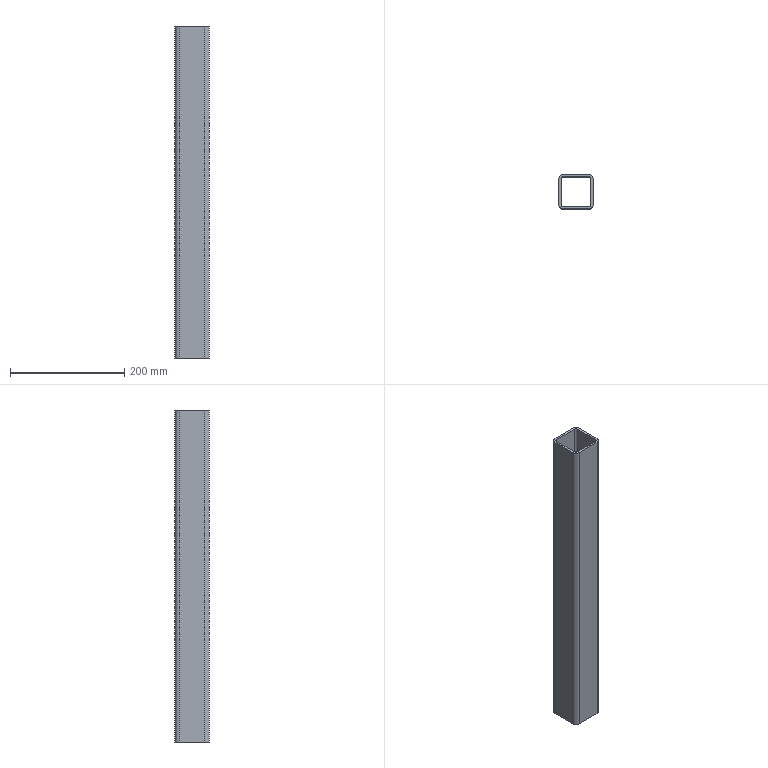Part | SolidWorks | features BaseBody 1 | 1 solid | 18 faces | box 60 x 60 x 580 mm | volume 495782 mm3 | plane 10 | cylinder 8 | commonest cylinder face diameters 8 x4 16 x4
STEP:
#1=CARTESIAN_POINT('',(-692.,1216.,-1300.));
#2=VERTEX_POINT('',#1);
#3=CARTESIAN_POINT('',(-692.,1216.,-720.));
#4=VERTEX_POINT('',#3);
#5=CARTESIAN_POINT('',(-692.,1216.,530.));
#6=DIRECTION('',(0.,0.,1.));
#7=VECTOR('',#6,1000.);
#8=LINE('',#5,#7);
#9=EDGE_CURVE('',#2,#4,#8,.T.);
#10=ORIENTED_EDGE('',*,*,#9,.T.);
#11=CARTESIAN_POINT('',(-648.,1216.,-720.));
#12=VERTEX_POINT('',#11);
#13=CARTESIAN_POINT('',(-692.,1216.,-720.));
#14=DIRECTION('',(1.,0.,0.));
#15=VECTOR('',#14,1000.);
#16=LINE('',#13,#15);
#17=EDGE_CURVE('',#4,#12,#16,.T.);
#18=ORIENTED_EDGE('',*,*,#17,.T.);
#19=CARTESIAN_POINT('',(-648.,1216.,-1300.));
#20=VERTEX_POINT('',#19);
#21=CARTESIAN_POINT('',(-648.,1216.,530.));
#22=DIRECTION('',(0.,0.,-1.));
#23=VECTOR('',#22,1000.);
#24=LINE('',#21,#23);
#25=EDGE_CURVE('',#12,#20,#24,.T.);
#26=ORIENTED_EDGE('',*,*,#25,.T.);
#27=CARTESIAN_POINT('',(-692.,1216.,-1300.));
#28=DIRECTION('',(-1.,0.,0.));
#29=VECTOR('',#28,1000.);
#30=LINE('',#27,#29);
#31=EDGE_CURVE('',#20,#2,#30,.T.);
#32=ORIENTED_EDGE('',*,*,#31,.T.);
#33=EDGE_LOOP('',(#10,#18,#26,#32));
#34=FACE_OUTER_BOUND('',#33,.T.);
#35=CARTESIAN_POINT('',(-692.,1216.,530.));
#36=DIRECTION('',(0.,1.,0.));
#37=DIRECTION('',(0.,0.,1.));
#38=AXIS2_PLACEMENT_3D('',#35,#36,#37);
#39=PLANE('',#38);
#40=ADVANCED_FACE('',(#34),#39,.T.);
#41=CARTESIAN_POINT('',(-696.,1220.,-720.));
#42=VERTEX_POINT('',#41);
#43=CARTESIAN_POINT('',(-692.,1220.,-720.));
#44=DIRECTION('',(0.,0.,1.));
#45=DIRECTION('',(-1.,0.,0.));
#46=AXIS2_PLACEMENT_3D('',#43,#44,#45);
#47=CIRCLE('',#46,4.);
#48=EDGE_CURVE('',#42,#4,#47,.T.);
#49=ORIENTED_EDGE('',*,*,#48,.F.);
#50=CARTESIAN_POINT('',(-696.,1264.,-720.));
#51=VERTEX_POINT('',#50);
#52=CARTESIAN_POINT('',(-696.,1242.,-720.));
#53=DIRECTION('',(0.,-1.,0.));
#54=VECTOR('',#53,1000.);
#55=LINE('',#52,#54);
#56=EDGE_CURVE('',#51,#42,#55,.T.);
#57=ORIENTED_EDGE('',*,*,#56,.F.);
#58=CARTESIAN_POINT('',(-692.,1268.,-720.));
#59=VERTEX_POINT('',#58);
#60=CARTESIAN_POINT('',(-692.,1264.,-720.));
#61=DIRECTION('',(0.,0.,1.));
#62=DIRECTION('',(-1.,0.,0.));
#63=AXIS2_PLACEMENT_3D('',#60,#61,#62);
#64=CIRCLE('',#63,4.);
#65=EDGE_CURVE('',#59,#51,#64,.T.);
#66=ORIENTED_EDGE('',*,*,#65,.F.);
#67=CARTESIAN_POINT('',(-648.,1268.,-720.));
#68=VERTEX_POINT('',#67);
#69=CARTESIAN_POINT('',(0.,1268.,-720.));
#70=DIRECTION('',(-1.,0.,0.));
#71=VECTOR('',#70,1000.);
#72=LINE('',#69,#71);
#73=EDGE_CURVE('',#68,#59,#72,.T.);
#74=ORIENTED_EDGE('',*,*,#73,.F.);
#75=CARTESIAN_POINT('',(-644.,1264.,-720.));
#76=VERTEX_POINT('',#75);
#77=CARTESIAN_POINT('',(-648.,1264.,-720.));
#78=DIRECTION('',(0.,0.,1.));
#79=DIRECTION('',(-1.,0.,0.));
#80=AXIS2_PLACEMENT_3D('',#77,#78,#79);
#81=CIRCLE('',#80,4.);
#82=EDGE_CURVE('',#76,#68,#81,.T.);
#83=ORIENTED_EDGE('',*,*,#82,.F.);
#84=CARTESIAN_POINT('',(-644.,1220.,-720.));
#85=VERTEX_POINT('',#84);
#86=CARTESIAN_POINT('',(-644.,1242.,-720.));
#87=DIRECTION('',(0.,1.,0.));
#88=VECTOR('',#87,1000.);
#89=LINE('',#86,#88);
#90=EDGE_CURVE('',#85,#76,#89,.T.);
#91=ORIENTED_EDGE('',*,*,#90,.F.);
#92=CARTESIAN_POINT('',(-648.,1220.,-720.));
#93=DIRECTION('',(0.,0.,1.));
#94=DIRECTION('',(-1.,0.,0.));
#95=AXIS2_PLACEMENT_3D('',#92,#93,#94);
#96=CIRCLE('',#95,4.);
#97=EDGE_CURVE('',#12,#85,#96,.T.);
#98=ORIENTED_EDGE('',*,*,#97,.F.);
#99=ORIENTED_EDGE('',*,*,#17,.F.);
#100=EDGE_LOOP('',(#49,#57,#66,#74,#83,#91,#98,#99));
#101=FACE_BOUND('',#100,.T.);
#102=CARTESIAN_POINT('',(-640.,1264.,-720.));
#103=VERTEX_POINT('',#102);
#104=CARTESIAN_POINT('',(-640.,1220.,-720.));
#105=VERTEX_POINT('',#104);
#106=CARTESIAN_POINT('',(-640.,1242.,-720.));
#107=DIRECTION('',(0.,-1.,0.));
#108=VECTOR('',#107,1000.);
#109=LINE('',#106,#108);
#110=EDGE_CURVE('',#103,#105,#109,.T.);
#111=ORIENTED_EDGE('',*,*,#110,.F.);
#112=CARTESIAN_POINT('',(-648.,1272.,-720.));
#113=VERTEX_POINT('',#112);
#114=CARTESIAN_POINT('',(-648.,1264.,-720.));
#115=DIRECTION('',(0.,0.,-1.));
#116=DIRECTION('',(-1.,0.,0.));
#117=AXIS2_PLACEMENT_3D('',#114,#115,#116);
#118=CIRCLE('',#117,8.);
#119=EDGE_CURVE('',#113,#103,#118,.T.);
#120=ORIENTED_EDGE('',*,*,#119,.F.);
#121=CARTESIAN_POINT('',(-692.,1272.,-720.));
#122=VERTEX_POINT('',#121);
#123=CARTESIAN_POINT('',(0.,1272.,-720.));
#124=DIRECTION('',(1.,0.,0.));
#125=VECTOR('',#124,1000.);
#126=LINE('',#123,#125);
#127=EDGE_CURVE('',#122,#113,#126,.T.);
#128=ORIENTED_EDGE('',*,*,#127,.F.);
#129=CARTESIAN_POINT('',(-700.,1264.,-720.));
#130=VERTEX_POINT('',#129);
#131=CARTESIAN_POINT('',(-692.,1264.,-720.));
#132=DIRECTION('',(0.,0.,-1.));
#133=DIRECTION('',(-1.,0.,0.));
#134=AXIS2_PLACEMENT_3D('',#131,#132,#133);
#135=CIRCLE('',#134,8.);
#136=EDGE_CURVE('',#130,#122,#135,.T.);
#137=ORIENTED_EDGE('',*,*,#136,.F.);
#138=CARTESIAN_POINT('',(-700.,1220.,-720.));
#139=VERTEX_POINT('',#138);
#140=CARTESIAN_POINT('',(-700.,1242.,-720.));
#141=DIRECTION('',(0.,1.,0.));
#142=VECTOR('',#141,1000.);
#143=LINE('',#140,#142);
#144=EDGE_CURVE('',#139,#130,#143,.T.);
#145=ORIENTED_EDGE('',*,*,#144,.F.);
#146=CARTESIAN_POINT('',(-692.,1212.,-720.));
#147=VERTEX_POINT('',#146);
#148=CARTESIAN_POINT('',(-692.,1220.,-720.));
#149=DIRECTION('',(0.,0.,-1.));
#150=DIRECTION('',(-1.,0.,0.));
#151=AXIS2_PLACEMENT_3D('',#148,#149,#150);
#152=CIRCLE('',#151,8.);
#153=EDGE_CURVE('',#147,#139,#152,.T.);
#154=ORIENTED_EDGE('',*,*,#153,.F.);
#155=CARTESIAN_POINT('',(-648.,1212.,-720.));
#156=VERTEX_POINT('',#155);
#157=CARTESIAN_POINT('',(0.,1212.,-720.));
#158=DIRECTION('',(-1.,0.,0.));
#159=VECTOR('',#158,1000.);
#160=LINE('',#157,#159);
#161=EDGE_CURVE('',#156,#147,#160,.T.);
#162=ORIENTED_EDGE('',*,*,#161,.F.);
#163=CARTESIAN_POINT('',(-648.,1220.,-720.));
#164=DIRECTION('',(0.,0.,-1.));
#165=DIRECTION('',(-1.,0.,0.));
#166=AXIS2_PLACEMENT_3D('',#163,#164,#165);
#167=CIRCLE('',#166,8.);
#168=EDGE_CURVE('',#105,#156,#167,.T.);
#169=ORIENTED_EDGE('',*,*,#168,.F.);
#170=EDGE_LOOP('',(#111,#120,#128,#137,#145,#154,#162,#169));
#171=FACE_OUTER_BOUND('',#170,.T.);
#172=CARTESIAN_POINT('',(0.,1242.,-720.));
#173=DIRECTION('',(0.,0.,-1.));
#174=DIRECTION('',(-1.,0.,0.));
#175=AXIS2_PLACEMENT_3D('',#172,#173,#174);
#176=PLANE('',#175);
#177=ADVANCED_FACE('',(#101,#171),#176,.F.);
#178=CARTESIAN_POINT('',(-696.,1220.,-1300.));
#179=VERTEX_POINT('',#178);
#180=CARTESIAN_POINT('',(-692.,1220.,-1300.));
#181=DIRECTION('',(0.,0.,1.));
#182=DIRECTION('',(-1.,0.,0.));
#183=AXIS2_PLACEMENT_3D('',#180,#181,#182);
#184=CIRCLE('',#183,4.);
#185=EDGE_CURVE('',#179,#2,#184,.T.);
#186=ORIENTED_EDGE('',*,*,#185,.F.);
#187=CARTESIAN_POINT('',(-696.,1220.,530.));
#188=DIRECTION('',(0.,0.,-1.));
#189=VECTOR('',#188,1000.);
#190=LINE('',#187,#189);
#191=EDGE_CURVE('',#42,#179,#190,.T.);
#192=ORIENTED_EDGE('',*,*,#191,.F.);
#193=ORIENTED_EDGE('',*,*,#48,.T.);
#194=ORIENTED_EDGE('',*,*,#9,.F.);
#195=EDGE_LOOP('',(#186,#192,#193,#194));
#196=FACE_OUTER_BOUND('',#195,.T.);
#197=CARTESIAN_POINT('',(-692.,1220.,530.));
#198=DIRECTION('',(0.,0.,-1.));
#199=DIRECTION('',(-1.,0.,0.));
#200=AXIS2_PLACEMENT_3D('',#197,#198,#199);
#201=CYLINDRICAL_SURFACE('',#200,4.);
#202=ADVANCED_FACE('',(#196),#201,.F.);
#203=ORIENTED_EDGE('',*,*,#31,.F.);
#204=CARTESIAN_POINT('',(-644.,1220.,-1300.));
#205=VERTEX_POINT('',#204);
#206=CARTESIAN_POINT('',(-648.,1220.,-1300.));
#207=DIRECTION('',(0.,0.,1.));
#208=DIRECTION('',(-1.,0.,0.));
#209=AXIS2_PLACEMENT_3D('',#206,#207,#208);
#210=CIRCLE('',#209,4.);
#211=EDGE_CURVE('',#20,#205,#210,.T.);
#212=ORIENTED_EDGE('',*,*,#211,.T.);
#213=CARTESIAN_POINT('',(-644.,1264.,-1300.));
#214=VERTEX_POINT('',#213);
#215=CARTESIAN_POINT('',(-644.,1242.,-1300.));
#216=DIRECTION('',(0.,1.,0.));
#217=VECTOR('',#216,1000.);
#218=LINE('',#215,#217);
#219=EDGE_CURVE('',#205,#214,#218,.T.);
#220=ORIENTED_EDGE('',*,*,#219,.T.);
#221=CARTESIAN_POINT('',(-648.,1268.,-1300.));
#222=VERTEX_POINT('',#221);
#223=CARTESIAN_POINT('',(-648.,1264.,-1300.));
#224=DIRECTION('',(0.,0.,1.));
#225=DIRECTION('',(-1.,0.,0.));
#226=AXIS2_PLACEMENT_3D('',#223,#224,#225);
#227=CIRCLE('',#226,4.);
#228=EDGE_CURVE('',#214,#222,#227,.T.);
#229=ORIENTED_EDGE('',*,*,#228,.T.);
#230=CARTESIAN_POINT('',(-692.,1268.,-1300.));
#231=VERTEX_POINT('',#230);
#232=CARTESIAN_POINT('',(-700.,1268.,-1300.));
#233=DIRECTION('',(-1.,0.,0.));
#234=VECTOR('',#233,1000.);
#235=LINE('',#232,#234);
#236=EDGE_CURVE('',#222,#231,#235,.T.);
#237=ORIENTED_EDGE('',*,*,#236,.T.);
#238=CARTESIAN_POINT('',(-696.,1264.,-1300.));
#239=VERTEX_POINT('',#238);
#240=CARTESIAN_POINT('',(-692.,1264.,-1300.));
#241=DIRECTION('',(0.,0.,1.));
#242=DIRECTION('',(-1.,0.,0.));
#243=AXIS2_PLACEMENT_3D('',#240,#241,#242);
#244=CIRCLE('',#243,4.);
#245=EDGE_CURVE('',#231,#239,#244,.T.);
#246=ORIENTED_EDGE('',*,*,#245,.T.);
#247=CARTESIAN_POINT('',(-696.,1242.,-1300.));
#248=DIRECTION('',(0.,-1.,0.));
#249=VECTOR('',#248,1000.);
#250=LINE('',#247,#249);
#251=EDGE_CURVE('',#239,#179,#250,.T.);
#252=ORIENTED_EDGE('',*,*,#251,.T.);
#253=ORIENTED_EDGE('',*,*,#185,.T.);
#254=EDGE_LOOP('',(#203,#212,#220,#229,#237,#246,#252,#253));
#255=FACE_BOUND('',#254,.T.);
#256=CARTESIAN_POINT('',(-640.,1220.,-1300.));
#257=VERTEX_POINT('',#256);
#258=CARTESIAN_POINT('',(-648.,1212.,-1300.));
#259=VERTEX_POINT('',#258);
#260=CARTESIAN_POINT('',(-648.,1220.,-1300.));
#261=DIRECTION('',(0.,0.,-1.));
#262=DIRECTION('',(-1.,0.,0.));
#263=AXIS2_PLACEMENT_3D('',#260,#261,#262);
#264=CIRCLE('',#263,8.);
#265=EDGE_CURVE('',#257,#259,#264,.T.);
#266=ORIENTED_EDGE('',*,*,#265,.T.);
#267=CARTESIAN_POINT('',(-692.,1212.,-1300.));
#268=VERTEX_POINT('',#267);
#269=CARTESIAN_POINT('',(-700.,1212.,-1300.));
#270=DIRECTION('',(-1.,0.,0.));
#271=VECTOR('',#270,1000.);
#272=LINE('',#269,#271);
#273=EDGE_CURVE('',#259,#268,#272,.T.);
#274=ORIENTED_EDGE('',*,*,#273,.T.);
#275=CARTESIAN_POINT('',(-700.,1220.,-1300.));
#276=VERTEX_POINT('',#275);
#277=CARTESIAN_POINT('',(-692.,1220.,-1300.));
#278=DIRECTION('',(0.,0.,-1.));
#279=DIRECTION('',(-1.,0.,0.));
#280=AXIS2_PLACEMENT_3D('',#277,#278,#279);
#281=CIRCLE('',#280,8.);
#282=EDGE_CURVE('',#268,#276,#281,.T.);
#283=ORIENTED_EDGE('',*,*,#282,.T.);
#284=CARTESIAN_POINT('',(-700.,1264.,-1300.));
#285=VERTEX_POINT('',#284);
#286=CARTESIAN_POINT('',(-700.,1242.,-1300.));
#287=DIRECTION('',(0.,1.,0.));
#288=VECTOR('',#287,1000.);
#289=LINE('',#286,#288);
#290=EDGE_CURVE('',#276,#285,#289,.T.);
#291=ORIENTED_EDGE('',*,*,#290,.T.);
#292=CARTESIAN_POINT('',(-692.,1272.,-1300.));
#293=VERTEX_POINT('',#292);
#294=CARTESIAN_POINT('',(-692.,1264.,-1300.));
#295=DIRECTION('',(0.,0.,-1.));
#296=DIRECTION('',(-1.,0.,0.));
#297=AXIS2_PLACEMENT_3D('',#294,#295,#296);
#298=CIRCLE('',#297,8.);
#299=EDGE_CURVE('',#285,#293,#298,.T.);
#300=ORIENTED_EDGE('',*,*,#299,.T.);
#301=CARTESIAN_POINT('',(-648.,1272.,-1300.));
#302=VERTEX_POINT('',#301);
#303=CARTESIAN_POINT('',(-700.,1272.,-1300.));
#304=DIRECTION('',(1.,0.,0.));
#305=VECTOR('',#304,1000.);
#306=LINE('',#303,#305);
#307=EDGE_CURVE('',#293,#302,#306,.T.);
#308=ORIENTED_EDGE('',*,*,#307,.T.);
#309=CARTESIAN_POINT('',(-640.,1264.,-1300.));
#310=VERTEX_POINT('',#309);
#311=CARTESIAN_POINT('',(-648.,1264.,-1300.));
#312=DIRECTION('',(0.,0.,-1.));
#313=DIRECTION('',(-1.,0.,0.));
#314=AXIS2_PLACEMENT_3D('',#311,#312,#313);
#315=CIRCLE('',#314,8.);
#316=EDGE_CURVE('',#302,#310,#315,.T.);
#317=ORIENTED_EDGE('',*,*,#316,.T.);
#318=CARTESIAN_POINT('',(-640.,1242.,-1300.));
#319=DIRECTION('',(0.,-1.,0.));
#320=VECTOR('',#319,1000.);
#321=LINE('',#318,#320);
#322=EDGE_CURVE('',#310,#257,#321,.T.);
#323=ORIENTED_EDGE('',*,*,#322,.T.);
#324=EDGE_LOOP('',(#266,#274,#283,#291,#300,#308,#317,#323));
#325=FACE_OUTER_BOUND('',#324,.T.);
#326=CARTESIAN_POINT('',(-700.,1242.,-1300.));
#327=DIRECTION('',(0.,0.,-1.));
#328=DIRECTION('',(-1.,0.,0.));
#329=AXIS2_PLACEMENT_3D('',#326,#327,#328);
#330=PLANE('',#329);
#331=ADVANCED_FACE('',(#255,#325),#330,.T.);
#332=ORIENTED_EDGE('',*,*,#211,.F.);
#333=ORIENTED_EDGE('',*,*,#25,.F.);
#334=ORIENTED_EDGE('',*,*,#97,.T.);
#335=CARTESIAN_POINT('',(-644.,1220.,530.));
#336=DIRECTION('',(0.,0.,1.));
#337=VECTOR('',#336,1000.);
#338=LINE('',#335,#337);
#339=EDGE_CURVE('',#205,#85,#338,.T.);
#340=ORIENTED_EDGE('',*,*,#339,.F.);
#341=EDGE_LOOP('',(#332,#333,#334,#340));
#342=FACE_OUTER_BOUND('',#341,.T.);
#343=CARTESIAN_POINT('',(-648.,1220.,530.));
#344=DIRECTION('',(0.,0.,-1.));
#345=DIRECTION('',(-1.,0.,0.));
#346=AXIS2_PLACEMENT_3D('',#343,#344,#345);
#347=CYLINDRICAL_SURFACE('',#346,4.);
#348=ADVANCED_FACE('',(#342),#347,.F.);
#349=CARTESIAN_POINT('',(-696.,1264.,530.));
#350=DIRECTION('',(0.,0.,1.));
#351=VECTOR('',#350,1000.);
#352=LINE('',#349,#351);
#353=EDGE_CURVE('',#239,#51,#352,.T.);
#354=ORIENTED_EDGE('',*,*,#353,.T.);
#355=ORIENTED_EDGE('',*,*,#56,.T.);
#356=ORIENTED_EDGE('',*,*,#191,.T.);
#357=ORIENTED_EDGE('',*,*,#251,.F.);
#358=EDGE_LOOP('',(#354,#355,#356,#357));
#359=FACE_OUTER_BOUND('',#358,.T.);
#360=CARTESIAN_POINT('',(-696.,1220.,530.));
#361=DIRECTION('',(1.,0.,0.));
#362=DIRECTION('',(0.,0.,-1.));
#363=AXIS2_PLACEMENT_3D('',#360,#361,#362);
#364=PLANE('',#363);
#365=ADVANCED_FACE('',(#359),#364,.T.);
#366=ORIENTED_EDGE('',*,*,#245,.F.);
#367=CARTESIAN_POINT('',(-692.,1268.,530.));
#368=DIRECTION('',(0.,0.,-1.));
#369=VECTOR('',#368,1000.);
#370=LINE('',#367,#369);
#371=EDGE_CURVE('',#59,#231,#370,.T.);
#372=ORIENTED_EDGE('',*,*,#371,.F.);
#373=ORIENTED_EDGE('',*,*,#65,.T.);
#374=ORIENTED_EDGE('',*,*,#353,.F.);
#375=EDGE_LOOP('',(#366,#372,#373,#374));
#376=FACE_OUTER_BOUND('',#375,.T.);
#377=CARTESIAN_POINT('',(-692.,1264.,530.));
#378=DIRECTION('',(0.,0.,-1.));
#379=DIRECTION('',(-1.,0.,0.));
#380=AXIS2_PLACEMENT_3D('',#377,#378,#379);
#381=CYLINDRICAL_SURFACE('',#380,4.);
#382=ADVANCED_FACE('',(#376),#381,.F.);
#383=CARTESIAN_POINT('',(-648.,1268.,530.));
#384=DIRECTION('',(0.,0.,1.));
#385=VECTOR('',#384,1000.);
#386=LINE('',#383,#385);
#387=EDGE_CURVE('',#222,#68,#386,.T.);
#388=ORIENTED_EDGE('',*,*,#387,.T.);
#389=ORIENTED_EDGE('',*,*,#73,.T.);
#390=ORIENTED_EDGE('',*,*,#371,.T.);
#391=ORIENTED_EDGE('',*,*,#236,.F.);
#392=EDGE_LOOP('',(#388,#389,#390,#391));
#393=FACE_OUTER_BOUND('',#392,.T.);
#394=CARTESIAN_POINT('',(-648.,1268.,530.));
#395=DIRECTION('',(0.,-1.,0.));
#396=DIRECTION('',(0.,0.,-1.));
#397=AXIS2_PLACEMENT_3D('',#394,#395,#396);
#398=PLANE('',#397);
#399=ADVANCED_FACE('',(#393),#398,.T.);
#400=ORIENTED_EDGE('',*,*,#228,.F.);
#401=CARTESIAN_POINT('',(-644.,1264.,530.));
#402=DIRECTION('',(0.,0.,-1.));
#403=VECTOR('',#402,1000.);
#404=LINE('',#401,#403);
#405=EDGE_CURVE('',#76,#214,#404,.T.);
#406=ORIENTED_EDGE('',*,*,#405,.F.);
#407=ORIENTED_EDGE('',*,*,#82,.T.);
#408=ORIENTED_EDGE('',*,*,#387,.F.);
#409=EDGE_LOOP('',(#400,#406,#407,#408));
#410=FACE_OUTER_BOUND('',#409,.T.);
#411=CARTESIAN_POINT('',(-648.,1264.,530.));
#412=DIRECTION('',(0.,0.,-1.));
#413=DIRECTION('',(-1.,0.,0.));
#414=AXIS2_PLACEMENT_3D('',#411,#412,#413);
#415=CYLINDRICAL_SURFACE('',#414,4.);
#416=ADVANCED_FACE('',(#410),#415,.F.);
#417=ORIENTED_EDGE('',*,*,#339,.T.);
#418=ORIENTED_EDGE('',*,*,#90,.T.);
#419=ORIENTED_EDGE('',*,*,#405,.T.);
#420=ORIENTED_EDGE('',*,*,#219,.F.);
#421=EDGE_LOOP('',(#417,#418,#419,#420));
#422=FACE_OUTER_BOUND('',#421,.T.);
#423=CARTESIAN_POINT('',(-644.,1264.,530.));
#424=DIRECTION('',(-1.,0.,0.));
#425=DIRECTION('',(0.,0.,1.));
#426=AXIS2_PLACEMENT_3D('',#423,#424,#425);
#427=PLANE('',#426);
#428=ADVANCED_FACE('',(#422),#427,.T.);
#429=ORIENTED_EDGE('',*,*,#265,.F.);
#430=CARTESIAN_POINT('',(-640.,1220.,530.));
#431=DIRECTION('',(0.,0.,1.));
#432=VECTOR('',#431,1000.);
#433=LINE('',#430,#432);
#434=EDGE_CURVE('',#257,#105,#433,.T.);
#435=ORIENTED_EDGE('',*,*,#434,.T.);
#436=ORIENTED_EDGE('',*,*,#168,.T.);
#437=CARTESIAN_POINT('',(-648.,1212.,530.));
#438=DIRECTION('',(0.,0.,-1.));
#439=VECTOR('',#438,1000.);
#440=LINE('',#437,#439);
#441=EDGE_CURVE('',#156,#259,#440,.T.);
#442=ORIENTED_EDGE('',*,*,#441,.T.);
#443=EDGE_LOOP('',(#429,#435,#436,#442));
#444=FACE_OUTER_BOUND('',#443,.T.);
#445=CARTESIAN_POINT('',(-648.,1220.,530.));
#446=DIRECTION('',(0.,0.,-1.));
#447=DIRECTION('',(-1.,0.,0.));
#448=AXIS2_PLACEMENT_3D('',#445,#446,#447);
#449=CYLINDRICAL_SURFACE('',#448,8.);
#450=ADVANCED_FACE('',(#444),#449,.T.);
#451=ORIENTED_EDGE('',*,*,#434,.F.);
#452=ORIENTED_EDGE('',*,*,#322,.F.);
#453=CARTESIAN_POINT('',(-640.,1264.,530.));
#454=DIRECTION('',(0.,0.,-1.));
#455=VECTOR('',#454,1000.);
#456=LINE('',#453,#455);
#457=EDGE_CURVE('',#103,#310,#456,.T.);
#458=ORIENTED_EDGE('',*,*,#457,.F.);
#459=ORIENTED_EDGE('',*,*,#110,.T.);
#460=EDGE_LOOP('',(#451,#452,#458,#459));
#461=FACE_OUTER_BOUND('',#460,.T.);
#462=CARTESIAN_POINT('',(-640.,1264.,530.));
#463=DIRECTION('',(-1.,0.,0.));
#464=DIRECTION('',(0.,0.,1.));
#465=AXIS2_PLACEMENT_3D('',#462,#463,#464);
#466=PLANE('',#465);
#467=ADVANCED_FACE('',(#461),#466,.F.);
#468=ORIENTED_EDGE('',*,*,#316,.F.);
#469=CARTESIAN_POINT('',(-648.,1272.,530.));
#470=DIRECTION('',(0.,0.,1.));
#471=VECTOR('',#470,1000.);
#472=LINE('',#469,#471);
#473=EDGE_CURVE('',#302,#113,#472,.T.);
#474=ORIENTED_EDGE('',*,*,#473,.T.);
#475=ORIENTED_EDGE('',*,*,#119,.T.);
#476=ORIENTED_EDGE('',*,*,#457,.T.);
#477=EDGE_LOOP('',(#468,#474,#475,#476));
#478=FACE_OUTER_BOUND('',#477,.T.);
#479=CARTESIAN_POINT('',(-648.,1264.,530.));
#480=DIRECTION('',(0.,0.,-1.));
#481=DIRECTION('',(-1.,0.,0.));
#482=AXIS2_PLACEMENT_3D('',#479,#480,#481);
#483=CYLINDRICAL_SURFACE('',#482,8.);
#484=ADVANCED_FACE('',(#478),#483,.T.);
#485=ORIENTED_EDGE('',*,*,#473,.F.);
#486=ORIENTED_EDGE('',*,*,#307,.F.);
#487=CARTESIAN_POINT('',(-692.,1272.,530.));
#488=DIRECTION('',(0.,0.,-1.));
#489=VECTOR('',#488,1000.);
#490=LINE('',#487,#489);
#491=EDGE_CURVE('',#122,#293,#490,.T.);
#492=ORIENTED_EDGE('',*,*,#491,.F.);
#493=ORIENTED_EDGE('',*,*,#127,.T.);
#494=EDGE_LOOP('',(#485,#486,#492,#493));
#495=FACE_OUTER_BOUND('',#494,.T.);
#496=CARTESIAN_POINT('',(-648.,1272.,530.));
#497=DIRECTION('',(0.,-1.,0.));
#498=DIRECTION('',(0.,0.,-1.));
#499=AXIS2_PLACEMENT_3D('',#496,#497,#498);
#500=PLANE('',#499);
#501=ADVANCED_FACE('',(#495),#500,.F.);
#502=ORIENTED_EDGE('',*,*,#299,.F.);
#503=CARTESIAN_POINT('',(-700.,1264.,530.));
#504=DIRECTION('',(0.,0.,1.));
#505=VECTOR('',#504,1000.);
#506=LINE('',#503,#505);
#507=EDGE_CURVE('',#285,#130,#506,.T.);
#508=ORIENTED_EDGE('',*,*,#507,.T.);
#509=ORIENTED_EDGE('',*,*,#136,.T.);
#510=ORIENTED_EDGE('',*,*,#491,.T.);
#511=EDGE_LOOP('',(#502,#508,#509,#510));
#512=FACE_OUTER_BOUND('',#511,.T.);
#513=CARTESIAN_POINT('',(-692.,1264.,530.));
#514=DIRECTION('',(0.,0.,-1.));
#515=DIRECTION('',(-1.,0.,0.));
#516=AXIS2_PLACEMENT_3D('',#513,#514,#515);
#517=CYLINDRICAL_SURFACE('',#516,8.);
#518=ADVANCED_FACE('',(#512),#517,.T.);
#519=ORIENTED_EDGE('',*,*,#507,.F.);
#520=ORIENTED_EDGE('',*,*,#290,.F.);
#521=CARTESIAN_POINT('',(-700.,1220.,530.));
#522=DIRECTION('',(0.,0.,-1.));
#523=VECTOR('',#522,1000.);
#524=LINE('',#521,#523);
#525=EDGE_CURVE('',#139,#276,#524,.T.);
#526=ORIENTED_EDGE('',*,*,#525,.F.);
#527=ORIENTED_EDGE('',*,*,#144,.T.);
#528=EDGE_LOOP('',(#519,#520,#526,#527));
#529=FACE_OUTER_BOUND('',#528,.T.);
#530=CARTESIAN_POINT('',(-700.,1220.,530.));
#531=DIRECTION('',(1.,0.,0.));
#532=DIRECTION('',(0.,0.,-1.));
#533=AXIS2_PLACEMENT_3D('',#530,#531,#532);
#534=PLANE('',#533);
#535=ADVANCED_FACE('',(#529),#534,.F.);
#536=ORIENTED_EDGE('',*,*,#282,.F.);
#537=CARTESIAN_POINT('',(-692.,1212.,530.));
#538=DIRECTION('',(0.,0.,1.));
#539=VECTOR('',#538,1000.);
#540=LINE('',#537,#539);
#541=EDGE_CURVE('',#268,#147,#540,.T.);
#542=ORIENTED_EDGE('',*,*,#541,.T.);
#543=ORIENTED_EDGE('',*,*,#153,.T.);
#544=ORIENTED_EDGE('',*,*,#525,.T.);
#545=EDGE_LOOP('',(#536,#542,#543,#544));
#546=FACE_OUTER_BOUND('',#545,.T.);
#547=CARTESIAN_POINT('',(-692.,1220.,530.));
#548=DIRECTION('',(0.,0.,-1.));
#549=DIRECTION('',(-1.,0.,0.));
#550=AXIS2_PLACEMENT_3D('',#547,#548,#549);
#551=CYLINDRICAL_SURFACE('',#550,8.);
#552=ADVANCED_FACE('',(#546),#551,.T.);
#553=ORIENTED_EDGE('',*,*,#541,.F.);
#554=ORIENTED_EDGE('',*,*,#273,.F.);
#555=ORIENTED_EDGE('',*,*,#441,.F.);
#556=ORIENTED_EDGE('',*,*,#161,.T.);
#557=EDGE_LOOP('',(#553,#554,#555,#556));
#558=FACE_OUTER_BOUND('',#557,.T.);
#559=CARTESIAN_POINT('',(-692.,1212.,530.));
#560=DIRECTION('',(0.,1.,0.));
#561=DIRECTION('',(0.,0.,1.));
#562=AXIS2_PLACEMENT_3D('',#559,#560,#561);
#563=PLANE('',#562);
#564=ADVANCED_FACE('',(#558),#563,.F.);
#565=CLOSED_SHELL('',(#40,#177,#202,#331,#348,#365,#382,#399,#416,#428,#450,#467,#484,#501,#518,#535,#552,#564));
#566=MANIFOLD_SOLID_BREP('',#565);
#567=CARTESIAN_POINT('',(0.,0.,0.));
#568=DIRECTION('',(0.,0.,1.));
#569=DIRECTION('',(1.,0.,0.));
#570=AXIS2_PLACEMENT_3D('',#567,#568,#569);
#571=(LENGTH_UNIT()NAMED_UNIT(*)SI_UNIT(.MILLI.,.METRE.));
#572=UNCERTAINTY_MEASURE_WITH_UNIT(LENGTH_MEASURE(0.00001),#571,'','');
#573=(NAMED_UNIT(*)PLANE_ANGLE_UNIT()SI_UNIT($,.RADIAN.));
#574=(NAMED_UNIT(*)SI_UNIT($,.STERADIAN.)SOLID_ANGLE_UNIT());
#575=(GEOMETRIC_REPRESENTATION_CONTEXT(3)GLOBAL_UNCERTAINTY_ASSIGNED_CONTEXT((#572))GLOBAL_UNIT_ASSIGNED_CONTEXT((#571,#573,#574))REPRESENTATION_CONTEXT('',''));
#576=ADVANCED_BREP_SHAPE_REPRESENTATION('',(#566,#570),#575);